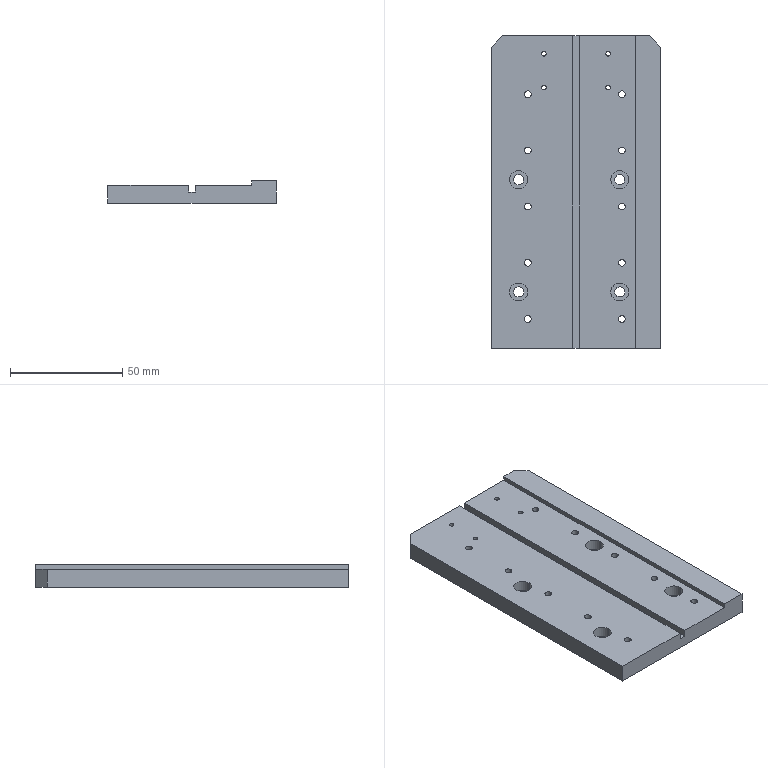Part | STEP file | ASND-0110-相机连接件2 | 1 solid | 62 faces | box 75 x 139 x 10 mm | volume 83120 mm3 | cylinder 44 | plane 18 | commonest cylinder face diameters 3 x20 2 x8 4.5 x8 8 x8